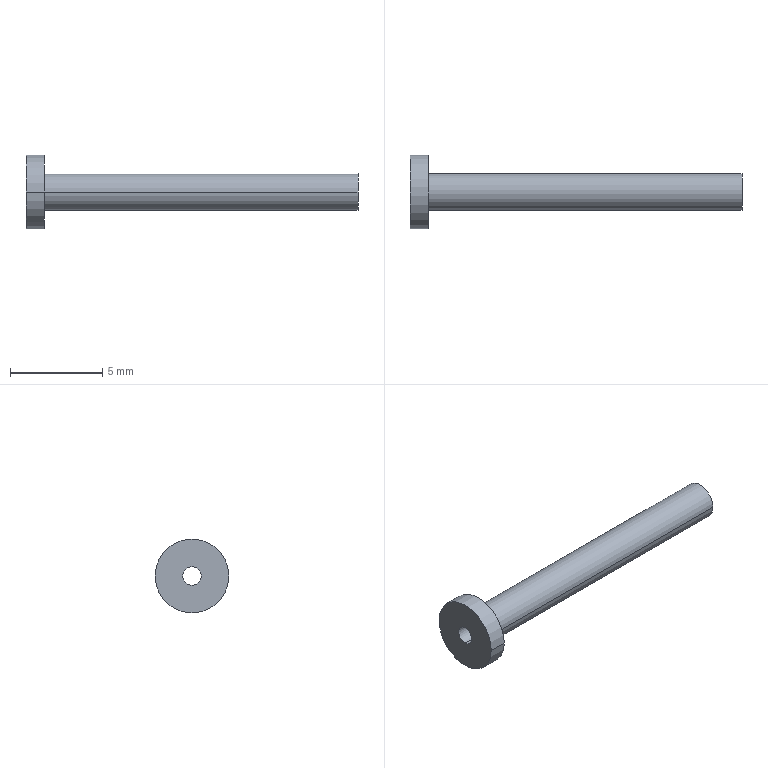Part | STEP file | SKITK4-8 | 1 solid | 9 faces | box 18 x 4 x 4 mm | volume 51.836 mm3 | cylinder 6 | plane 3 | commonest cylinder face diameters 1 x2 2 x2 4 x2
STEP:
#1=CARTESIAN_POINT('',(0.,0.,0.));
#2=DIRECTION('',(0.,0.,1.));
#3=DIRECTION('',(1.,0.,0.));
#4=AXIS2_PLACEMENT_3D('',#1,#2,#3);
#5=CARTESIAN_POINT('',(0.,0.,-0.5));
#6=VERTEX_POINT('',#5);
#7=CARTESIAN_POINT('',(18.,0.,-0.5));
#8=VERTEX_POINT('',#7);
#9=CARTESIAN_POINT('',(0.,0.,-0.5));
#10=DIRECTION('',(1.,0.,0.));
#11=VECTOR('',#10,1.);
#12=LINE('',#9,#11);
#13=CARTESIAN_POINT('',(0.,0.,0.));
#14=DIRECTION('',(1.,0.,0.));
#15=DIRECTION('',(0.,0.,-1.));
#16=AXIS2_PLACEMENT_3D('',#13,#14,#15);
#17=CYLINDRICAL_SURFACE('',#16,0.5);
#18=CARTESIAN_POINT('',(6.283,0.));
#19=DIRECTION('',(0.,1.));
#20=VECTOR('',#19,1.);
#21=LINE('',#18,#20);
#22=(GEOMETRIC_REPRESENTATION_CONTEXT(2)PARAMETRIC_REPRESENTATION_CONTEXT()REPRESENTATION_CONTEXT('',''));
#23=DEFINITIONAL_REPRESENTATION('',(#21),#22);
#24=PCURVE('',#17,#23);
#25=CARTESIAN_POINT('',(0.,0.,0.));
#26=DIRECTION('',(1.,0.,0.));
#27=DIRECTION('',(0.,0.,-1.));
#28=AXIS2_PLACEMENT_3D('',#25,#26,#27);
#29=CYLINDRICAL_SURFACE('',#28,0.5);
#30=CARTESIAN_POINT('',(0.,0.));
#31=DIRECTION('',(0.,1.));
#32=VECTOR('',#31,1.);
#33=LINE('',#30,#32);
#34=(GEOMETRIC_REPRESENTATION_CONTEXT(2)PARAMETRIC_REPRESENTATION_CONTEXT()REPRESENTATION_CONTEXT('',''));
#35=DEFINITIONAL_REPRESENTATION('',(#33),#34);
#36=PCURVE('',#29,#35);
#37=SURFACE_CURVE('',#12,(#24,#36),.PCURVE_S1.);
#38=EDGE_CURVE('',#6,#8,#37,.T.);
#39=ORIENTED_EDGE('',*,*,#38,.T.);
#40=CARTESIAN_POINT('',(18.,0.,0.5));
#41=VERTEX_POINT('',#40);
#42=CARTESIAN_POINT('',(18.,0.,0.));
#43=DIRECTION('',(-1.,0.,0.));
#44=DIRECTION('',(0.,0.,1.));
#45=AXIS2_PLACEMENT_3D('',#42,#43,#44);
#46=CIRCLE('',#45,0.5);
#47=CARTESIAN_POINT('',(9.425,18.));
#48=DIRECTION('',(-1.,0.));
#49=VECTOR('',#48,1.);
#50=LINE('',#47,#49);
#51=(GEOMETRIC_REPRESENTATION_CONTEXT(2)PARAMETRIC_REPRESENTATION_CONTEXT()REPRESENTATION_CONTEXT('',''));
#52=DEFINITIONAL_REPRESENTATION('',(#50),#51);
#53=PCURVE('',#17,#52);
#54=CARTESIAN_POINT('',(18.,0.,0.));
#55=DIRECTION('',(1.,0.,0.));
#56=DIRECTION('',(0.,1.,0.));
#57=AXIS2_PLACEMENT_3D('',#54,#55,#56);
#58=PLANE('',#57);
#59=CARTESIAN_POINT('',(0.,0.5));
#60=CARTESIAN_POINT('',(0.866,0.5));
#61=CARTESIAN_POINT('',(0.433,-0.25));
#62=CARTESIAN_POINT('',(0.,-1.));
#63=CARTESIAN_POINT('',(-0.433,-0.25));
#64=CARTESIAN_POINT('',(-0.866,0.5));
#65=CARTESIAN_POINT('',(0.,0.5));
#66=(BOUNDED_CURVE()B_SPLINE_CURVE(2,(#59,#60,#61,#62,#63,#64,#65),.UNSPECIFIED.,.T.,.F.)B_SPLINE_CURVE_WITH_KNOTS((1,2,2,2,2,1),(-2.094,0.,2.094,4.189,6.283,8.378),.UNSPECIFIED.)CURVE()GEOMETRIC_REPRESENTATION_ITEM()RATIONAL_B_SPLINE_CURVE((1.,0.5,1.,0.5,1.,0.5,1.))REPRESENTATION_ITEM(''));
#67=(GEOMETRIC_REPRESENTATION_CONTEXT(2)PARAMETRIC_REPRESENTATION_CONTEXT()REPRESENTATION_CONTEXT('',''));
#68=DEFINITIONAL_REPRESENTATION('',(#66),#67);
#69=PCURVE('',#58,#68);
#70=SURFACE_CURVE('',#46,(#53,#69),.PCURVE_S1.);
#71=EDGE_CURVE('',#8,#41,#70,.T.);
#72=ORIENTED_EDGE('',*,*,#71,.T.);
#73=CARTESIAN_POINT('',(0.,0.,0.5));
#74=VERTEX_POINT('',#73);
#75=CARTESIAN_POINT('',(0.,0.,0.5));
#76=DIRECTION('',(1.,0.,0.));
#77=VECTOR('',#76,1.);
#78=LINE('',#75,#77);
#79=CARTESIAN_POINT('',(3.142,0.));
#80=DIRECTION('',(0.,1.));
#81=VECTOR('',#80,1.);
#82=LINE('',#79,#81);
#83=(GEOMETRIC_REPRESENTATION_CONTEXT(2)PARAMETRIC_REPRESENTATION_CONTEXT()REPRESENTATION_CONTEXT('',''));
#84=DEFINITIONAL_REPRESENTATION('',(#82),#83);
#85=PCURVE('',#17,#84);
#86=CARTESIAN_POINT('',(3.142,0.));
#87=DIRECTION('',(0.,1.));
#88=VECTOR('',#87,1.);
#89=LINE('',#86,#88);
#90=(GEOMETRIC_REPRESENTATION_CONTEXT(2)PARAMETRIC_REPRESENTATION_CONTEXT()REPRESENTATION_CONTEXT('',''));
#91=DEFINITIONAL_REPRESENTATION('',(#89),#90);
#92=PCURVE('',#29,#91);
#93=SURFACE_CURVE('',#78,(#85,#92),.PCURVE_S1.);
#94=EDGE_CURVE('',#74,#41,#93,.T.);
#95=ORIENTED_EDGE('',*,*,#94,.F.);
#96=CARTESIAN_POINT('',(0.,0.,0.));
#97=DIRECTION('',(1.,0.,0.));
#98=DIRECTION('',(0.,0.,-1.));
#99=AXIS2_PLACEMENT_3D('',#96,#97,#98);
#100=CIRCLE('',#99,0.5);
#101=CARTESIAN_POINT('',(0.,0.));
#102=DIRECTION('',(1.,0.));
#103=VECTOR('',#102,1.);
#104=LINE('',#101,#103);
#105=(GEOMETRIC_REPRESENTATION_CONTEXT(2)PARAMETRIC_REPRESENTATION_CONTEXT()REPRESENTATION_CONTEXT('',''));
#106=DEFINITIONAL_REPRESENTATION('',(#104),#105);
#107=PCURVE('',#17,#106);
#108=CARTESIAN_POINT('',(0.,0.,0.));
#109=DIRECTION('',(-1.,0.,0.));
#110=DIRECTION('',(0.,-1.,0.));
#111=AXIS2_PLACEMENT_3D('',#108,#109,#110);
#112=PLANE('',#111);
#113=CARTESIAN_POINT('',(0.,-0.5));
#114=CARTESIAN_POINT('',(-0.866,-0.5));
#115=CARTESIAN_POINT('',(-0.433,0.25));
#116=CARTESIAN_POINT('',(0.,1.));
#117=CARTESIAN_POINT('',(0.433,0.25));
#118=CARTESIAN_POINT('',(0.866,-0.5));
#119=CARTESIAN_POINT('',(0.,-0.5));
#120=(BOUNDED_CURVE()B_SPLINE_CURVE(2,(#113,#114,#115,#116,#117,#118,#119),.UNSPECIFIED.,.T.,.F.)B_SPLINE_CURVE_WITH_KNOTS((1,2,2,2,2,1),(-2.094,0.,2.094,4.189,6.283,8.378),.UNSPECIFIED.)CURVE()GEOMETRIC_REPRESENTATION_ITEM()RATIONAL_B_SPLINE_CURVE((1.,0.5,1.,0.5,1.,0.5,1.))REPRESENTATION_ITEM(''));
#121=(GEOMETRIC_REPRESENTATION_CONTEXT(2)PARAMETRIC_REPRESENTATION_CONTEXT()REPRESENTATION_CONTEXT('',''));
#122=DEFINITIONAL_REPRESENTATION('',(#120),#121);
#123=PCURVE('',#112,#122);
#124=SURFACE_CURVE('',#100,(#107,#123),.PCURVE_S1.);
#125=EDGE_CURVE('',#74,#6,#124,.T.);
#126=ORIENTED_EDGE('',*,*,#125,.T.);
#127=EDGE_LOOP('',(#39,#72,#95,#126));
#128=FACE_BOUND('',#127,.F.);
#129=ADVANCED_FACE('',(#128),#17,.F.);
#130=CARTESIAN_POINT('',(1.,1.,0.));
#131=VERTEX_POINT('',#130);
#132=CARTESIAN_POINT('',(1.,-1.,0.));
#133=VERTEX_POINT('',#132);
#134=CARTESIAN_POINT('',(1.,0.,0.));
#135=DIRECTION('',(1.,0.,0.));
#136=DIRECTION('',(0.,1.,0.));
#137=AXIS2_PLACEMENT_3D('',#134,#135,#136);
#138=CIRCLE('',#137,1.);
#139=CARTESIAN_POINT('',(1.,0.,0.));
#140=DIRECTION('',(1.,0.,0.));
#141=DIRECTION('',(0.,1.,0.));
#142=AXIS2_PLACEMENT_3D('',#139,#140,#141);
#143=CYLINDRICAL_SURFACE('',#142,1.);
#144=CARTESIAN_POINT('',(0.,0.));
#145=DIRECTION('',(1.,0.));
#146=VECTOR('',#145,1.);
#147=LINE('',#144,#146);
#148=(GEOMETRIC_REPRESENTATION_CONTEXT(2)PARAMETRIC_REPRESENTATION_CONTEXT()REPRESENTATION_CONTEXT('',''));
#149=DEFINITIONAL_REPRESENTATION('',(#147),#148);
#150=PCURVE('',#143,#149);
#151=CARTESIAN_POINT('',(1.,0.,0.));
#152=DIRECTION('',(1.,0.,0.));
#153=DIRECTION('',(0.,1.,0.));
#154=AXIS2_PLACEMENT_3D('',#151,#152,#153);
#155=PLANE('',#154);
#156=CARTESIAN_POINT('',(0.,0.));
#157=DIRECTION('',(1.,0.));
#158=AXIS2_PLACEMENT_2D('',#156,#157);
#159=CIRCLE('',#158,1.);
#160=(GEOMETRIC_REPRESENTATION_CONTEXT(2)PARAMETRIC_REPRESENTATION_CONTEXT()REPRESENTATION_CONTEXT('',''));
#161=DEFINITIONAL_REPRESENTATION('',(#159),#160);
#162=PCURVE('',#155,#161);
#163=SURFACE_CURVE('',#138,(#150,#162),.PCURVE_S1.);
#164=EDGE_CURVE('',#131,#133,#163,.T.);
#165=ORIENTED_EDGE('',*,*,#164,.T.);
#166=CARTESIAN_POINT('',(18.,-1.,0.));
#167=VERTEX_POINT('',#166);
#168=CARTESIAN_POINT('',(1.,-1.,0.));
#169=DIRECTION('',(1.,0.,0.));
#170=VECTOR('',#169,1.);
#171=LINE('',#168,#170);
#172=CARTESIAN_POINT('',(3.142,0.));
#173=DIRECTION('',(0.,1.));
#174=VECTOR('',#173,1.);
#175=LINE('',#172,#174);
#176=(GEOMETRIC_REPRESENTATION_CONTEXT(2)PARAMETRIC_REPRESENTATION_CONTEXT()REPRESENTATION_CONTEXT('',''));
#177=DEFINITIONAL_REPRESENTATION('',(#175),#176);
#178=PCURVE('',#143,#177);
#179=CARTESIAN_POINT('',(1.,0.,0.));
#180=DIRECTION('',(1.,0.,0.));
#181=DIRECTION('',(0.,1.,0.));
#182=AXIS2_PLACEMENT_3D('',#179,#180,#181);
#183=CYLINDRICAL_SURFACE('',#182,1.);
#184=CARTESIAN_POINT('',(3.142,0.));
#185=DIRECTION('',(0.,1.));
#186=VECTOR('',#185,1.);
#187=LINE('',#184,#186);
#188=(GEOMETRIC_REPRESENTATION_CONTEXT(2)PARAMETRIC_REPRESENTATION_CONTEXT()REPRESENTATION_CONTEXT('',''));
#189=DEFINITIONAL_REPRESENTATION('',(#187),#188);
#190=PCURVE('',#183,#189);
#191=SURFACE_CURVE('',#171,(#178,#190),.PCURVE_S1.);
#192=EDGE_CURVE('',#133,#167,#191,.T.);
#193=ORIENTED_EDGE('',*,*,#192,.T.);
#194=CARTESIAN_POINT('',(18.,1.,0.));
#195=VERTEX_POINT('',#194);
#196=CARTESIAN_POINT('',(18.,0.,0.));
#197=DIRECTION('',(-1.,0.,0.));
#198=DIRECTION('',(0.,-1.,0.));
#199=AXIS2_PLACEMENT_3D('',#196,#197,#198);
#200=CIRCLE('',#199,1.);
#201=CARTESIAN_POINT('',(3.142,17.));
#202=DIRECTION('',(-1.,0.));
#203=VECTOR('',#202,1.);
#204=LINE('',#201,#203);
#205=(GEOMETRIC_REPRESENTATION_CONTEXT(2)PARAMETRIC_REPRESENTATION_CONTEXT()REPRESENTATION_CONTEXT('',''));
#206=DEFINITIONAL_REPRESENTATION('',(#204),#205);
#207=PCURVE('',#143,#206);
#208=CARTESIAN_POINT('',(-1.,0.));
#209=CARTESIAN_POINT('',(-1.,1.732));
#210=CARTESIAN_POINT('',(0.5,0.866));
#211=CARTESIAN_POINT('',(2.,0.));
#212=CARTESIAN_POINT('',(0.5,-0.866));
#213=CARTESIAN_POINT('',(-1.,-1.732));
#214=CARTESIAN_POINT('',(-1.,0.));
#215=(BOUNDED_CURVE()B_SPLINE_CURVE(2,(#208,#209,#210,#211,#212,#213,#214),.UNSPECIFIED.,.T.,.F.)B_SPLINE_CURVE_WITH_KNOTS((1,2,2,2,2,1),(-2.094,0.,2.094,4.189,6.283,8.378),.UNSPECIFIED.)CURVE()GEOMETRIC_REPRESENTATION_ITEM()RATIONAL_B_SPLINE_CURVE((1.,0.5,1.,0.5,1.,0.5,1.))REPRESENTATION_ITEM(''));
#216=(GEOMETRIC_REPRESENTATION_CONTEXT(2)PARAMETRIC_REPRESENTATION_CONTEXT()REPRESENTATION_CONTEXT('',''));
#217=DEFINITIONAL_REPRESENTATION('',(#215),#216);
#218=PCURVE('',#58,#217);
#219=SURFACE_CURVE('',#200,(#207,#218),.PCURVE_S1.);
#220=EDGE_CURVE('',#167,#195,#219,.T.);
#221=ORIENTED_EDGE('',*,*,#220,.T.);
#222=CARTESIAN_POINT('',(1.,1.,0.));
#223=DIRECTION('',(1.,0.,0.));
#224=VECTOR('',#223,1.);
#225=LINE('',#222,#224);
#226=CARTESIAN_POINT('',(0.,0.));
#227=DIRECTION('',(0.,1.));
#228=VECTOR('',#227,1.);
#229=LINE('',#226,#228);
#230=(GEOMETRIC_REPRESENTATION_CONTEXT(2)PARAMETRIC_REPRESENTATION_CONTEXT()REPRESENTATION_CONTEXT('',''));
#231=DEFINITIONAL_REPRESENTATION('',(#229),#230);
#232=PCURVE('',#143,#231);
#233=CARTESIAN_POINT('',(6.283,0.));
#234=DIRECTION('',(0.,1.));
#235=VECTOR('',#234,1.);
#236=LINE('',#233,#235);
#237=(GEOMETRIC_REPRESENTATION_CONTEXT(2)PARAMETRIC_REPRESENTATION_CONTEXT()REPRESENTATION_CONTEXT('',''));
#238=DEFINITIONAL_REPRESENTATION('',(#236),#237);
#239=PCURVE('',#183,#238);
#240=SURFACE_CURVE('',#225,(#232,#239),.PCURVE_S1.);
#241=EDGE_CURVE('',#131,#195,#240,.T.);
#242=ORIENTED_EDGE('',*,*,#241,.F.);
#243=EDGE_LOOP('',(#165,#193,#221,#242));
#244=FACE_BOUND('',#243,.T.);
#245=ADVANCED_FACE('',(#244),#143,.T.);
#246=CARTESIAN_POINT('',(0.,2.,0.));
#247=VERTEX_POINT('',#246);
#248=CARTESIAN_POINT('',(0.,-2.,0.));
#249=VERTEX_POINT('',#248);
#250=CARTESIAN_POINT('',(0.,0.,0.));
#251=DIRECTION('',(1.,0.,0.));
#252=DIRECTION('',(0.,1.,0.));
#253=AXIS2_PLACEMENT_3D('',#250,#251,#252);
#254=CIRCLE('',#253,2.);
#255=CARTESIAN_POINT('',(0.,0.,0.));
#256=DIRECTION('',(1.,0.,0.));
#257=DIRECTION('',(0.,1.,0.));
#258=AXIS2_PLACEMENT_3D('',#255,#256,#257);
#259=CYLINDRICAL_SURFACE('',#258,2.);
#260=CARTESIAN_POINT('',(0.,0.));
#261=DIRECTION('',(1.,0.));
#262=VECTOR('',#261,1.);
#263=LINE('',#260,#262);
#264=(GEOMETRIC_REPRESENTATION_CONTEXT(2)PARAMETRIC_REPRESENTATION_CONTEXT()REPRESENTATION_CONTEXT('',''));
#265=DEFINITIONAL_REPRESENTATION('',(#263),#264);
#266=PCURVE('',#259,#265);
#267=CARTESIAN_POINT('',(-2.,0.));
#268=CARTESIAN_POINT('',(-2.,3.464));
#269=CARTESIAN_POINT('',(1.,1.732));
#270=CARTESIAN_POINT('',(4.,0.));
#271=CARTESIAN_POINT('',(1.,-1.732));
#272=CARTESIAN_POINT('',(-2.,-3.464));
#273=CARTESIAN_POINT('',(-2.,0.));
#274=(BOUNDED_CURVE()B_SPLINE_CURVE(2,(#267,#268,#269,#270,#271,#272,#273),.UNSPECIFIED.,.T.,.F.)B_SPLINE_CURVE_WITH_KNOTS((1,2,2,2,2,1),(-2.094,0.,2.094,4.189,6.283,8.378),.UNSPECIFIED.)CURVE()GEOMETRIC_REPRESENTATION_ITEM()RATIONAL_B_SPLINE_CURVE((1.,0.5,1.,0.5,1.,0.5,1.))REPRESENTATION_ITEM(''));
#275=(GEOMETRIC_REPRESENTATION_CONTEXT(2)PARAMETRIC_REPRESENTATION_CONTEXT()REPRESENTATION_CONTEXT('',''));
#276=DEFINITIONAL_REPRESENTATION('',(#274),#275);
#277=PCURVE('',#112,#276);
#278=SURFACE_CURVE('',#254,(#266,#277),.PCURVE_S1.);
#279=EDGE_CURVE('',#247,#249,#278,.T.);
#280=ORIENTED_EDGE('',*,*,#279,.T.);
#281=CARTESIAN_POINT('',(1.,-2.,0.));
#282=VERTEX_POINT('',#281);
#283=CARTESIAN_POINT('',(0.,-2.,0.));
#284=DIRECTION('',(1.,0.,0.));
#285=VECTOR('',#284,1.);
#286=LINE('',#283,#285);
#287=CARTESIAN_POINT('',(3.142,0.));
#288=DIRECTION('',(0.,1.));
#289=VECTOR('',#288,1.);
#290=LINE('',#287,#289);
#291=(GEOMETRIC_REPRESENTATION_CONTEXT(2)PARAMETRIC_REPRESENTATION_CONTEXT()REPRESENTATION_CONTEXT('',''));
#292=DEFINITIONAL_REPRESENTATION('',(#290),#291);
#293=PCURVE('',#259,#292);
#294=CARTESIAN_POINT('',(0.,0.,0.));
#295=DIRECTION('',(1.,0.,0.));
#296=DIRECTION('',(0.,1.,0.));
#297=AXIS2_PLACEMENT_3D('',#294,#295,#296);
#298=CYLINDRICAL_SURFACE('',#297,2.);
#299=CARTESIAN_POINT('',(3.142,0.));
#300=DIRECTION('',(0.,1.));
#301=VECTOR('',#300,1.);
#302=LINE('',#299,#301);
#303=(GEOMETRIC_REPRESENTATION_CONTEXT(2)PARAMETRIC_REPRESENTATION_CONTEXT()REPRESENTATION_CONTEXT('',''));
#304=DEFINITIONAL_REPRESENTATION('',(#302),#303);
#305=PCURVE('',#298,#304);
#306=SURFACE_CURVE('',#286,(#293,#305),.PCURVE_S1.);
#307=EDGE_CURVE('',#249,#282,#306,.T.);
#308=ORIENTED_EDGE('',*,*,#307,.T.);
#309=CARTESIAN_POINT('',(1.,2.,0.));
#310=VERTEX_POINT('',#309);
#311=CARTESIAN_POINT('',(1.,0.,0.));
#312=DIRECTION('',(-1.,0.,0.));
#313=DIRECTION('',(0.,-1.,0.));
#314=AXIS2_PLACEMENT_3D('',#311,#312,#313);
#315=CIRCLE('',#314,2.);
#316=CARTESIAN_POINT('',(3.142,1.));
#317=DIRECTION('',(-1.,0.));
#318=VECTOR('',#317,1.);
#319=LINE('',#316,#318);
#320=(GEOMETRIC_REPRESENTATION_CONTEXT(2)PARAMETRIC_REPRESENTATION_CONTEXT()REPRESENTATION_CONTEXT('',''));
#321=DEFINITIONAL_REPRESENTATION('',(#319),#320);
#322=PCURVE('',#259,#321);
#323=CARTESIAN_POINT('',(-2.,0.));
#324=CARTESIAN_POINT('',(-2.,3.464));
#325=CARTESIAN_POINT('',(1.,1.732));
#326=CARTESIAN_POINT('',(4.,0.));
#327=CARTESIAN_POINT('',(1.,-1.732));
#328=CARTESIAN_POINT('',(-2.,-3.464));
#329=CARTESIAN_POINT('',(-2.,0.));
#330=(BOUNDED_CURVE()B_SPLINE_CURVE(2,(#323,#324,#325,#326,#327,#328,#329),.UNSPECIFIED.,.T.,.F.)B_SPLINE_CURVE_WITH_KNOTS((1,2,2,2,2,1),(-2.094,0.,2.094,4.189,6.283,8.378),.UNSPECIFIED.)CURVE()GEOMETRIC_REPRESENTATION_ITEM()RATIONAL_B_SPLINE_CURVE((1.,0.5,1.,0.5,1.,0.5,1.))REPRESENTATION_ITEM(''));
#331=(GEOMETRIC_REPRESENTATION_CONTEXT(2)PARAMETRIC_REPRESENTATION_CONTEXT()REPRESENTATION_CONTEXT('',''));
#332=DEFINITIONAL_REPRESENTATION('',(#330),#331);
#333=PCURVE('',#155,#332);
#334=SURFACE_CURVE('',#315,(#322,#333),.PCURVE_S1.);
#335=EDGE_CURVE('',#282,#310,#334,.T.);
#336=ORIENTED_EDGE('',*,*,#335,.T.);
#337=CARTESIAN_POINT('',(0.,2.,0.));
#338=DIRECTION('',(1.,0.,0.));
#339=VECTOR('',#338,1.);
#340=LINE('',#337,#339);
#341=CARTESIAN_POINT('',(0.,0.));
#342=DIRECTION('',(0.,1.));
#343=VECTOR('',#342,1.);
#344=LINE('',#341,#343);
#345=(GEOMETRIC_REPRESENTATION_CONTEXT(2)PARAMETRIC_REPRESENTATION_CONTEXT()REPRESENTATION_CONTEXT('',''));
#346=DEFINITIONAL_REPRESENTATION('',(#344),#345);
#347=PCURVE('',#259,#346);
#348=CARTESIAN_POINT('',(6.283,0.));
#349=DIRECTION('',(0.,1.));
#350=VECTOR('',#349,1.);
#351=LINE('',#348,#350);
#352=(GEOMETRIC_REPRESENTATION_CONTEXT(2)PARAMETRIC_REPRESENTATION_CONTEXT()REPRESENTATION_CONTEXT('',''));
#353=DEFINITIONAL_REPRESENTATION('',(#351),#352);
#354=PCURVE('',#298,#353);
#355=SURFACE_CURVE('',#340,(#347,#354),.PCURVE_S1.);
#356=EDGE_CURVE('',#247,#310,#355,.T.);
#357=ORIENTED_EDGE('',*,*,#356,.F.);
#358=EDGE_LOOP('',(#280,#308,#336,#357));
#359=FACE_BOUND('',#358,.T.);
#360=ADVANCED_FACE('',(#359),#259,.T.);
#361=ORIENTED_EDGE('',*,*,#164,.F.);
#362=CARTESIAN_POINT('',(1.,0.,0.));
#363=DIRECTION('',(1.,0.,0.));
#364=DIRECTION('',(0.,1.,0.));
#365=AXIS2_PLACEMENT_3D('',#362,#363,#364);
#366=CIRCLE('',#365,1.);
#367=CARTESIAN_POINT('',(0.,0.));
#368=DIRECTION('',(1.,0.));
#369=AXIS2_PLACEMENT_2D('',#367,#368);
#370=CIRCLE('',#369,1.);
#371=(GEOMETRIC_REPRESENTATION_CONTEXT(2)PARAMETRIC_REPRESENTATION_CONTEXT()REPRESENTATION_CONTEXT('',''));
#372=DEFINITIONAL_REPRESENTATION('',(#370),#371);
#373=PCURVE('',#155,#372);
#374=CARTESIAN_POINT('',(0.,0.));
#375=DIRECTION('',(1.,0.));
#376=VECTOR('',#375,1.);
#377=LINE('',#374,#376);
#378=(GEOMETRIC_REPRESENTATION_CONTEXT(2)PARAMETRIC_REPRESENTATION_CONTEXT()REPRESENTATION_CONTEXT('',''));
#379=DEFINITIONAL_REPRESENTATION('',(#377),#378);
#380=PCURVE('',#183,#379);
#381=SURFACE_CURVE('',#366,(#373,#380),.PCURVE_S1.);
#382=EDGE_CURVE('',#133,#131,#381,.T.);
#383=ORIENTED_EDGE('',*,*,#382,.F.);
#384=EDGE_LOOP('',(#361,#383));
#385=FACE_BOUND('',#384,.T.);
#386=CARTESIAN_POINT('',(1.,0.,0.));
#387=DIRECTION('',(-1.,0.,0.));
#388=DIRECTION('',(0.,-1.,0.));
#389=AXIS2_PLACEMENT_3D('',#386,#387,#388);
#390=CIRCLE('',#389,2.);
#391=CARTESIAN_POINT('',(-2.,0.));
#392=CARTESIAN_POINT('',(-2.,3.464));
#393=CARTESIAN_POINT('',(1.,1.732));
#394=CARTESIAN_POINT('',(4.,0.));
#395=CARTESIAN_POINT('',(1.,-1.732));
#396=CARTESIAN_POINT('',(-2.,-3.464));
#397=CARTESIAN_POINT('',(-2.,0.));
#398=(BOUNDED_CURVE()B_SPLINE_CURVE(2,(#391,#392,#393,#394,#395,#396,#397),.UNSPECIFIED.,.T.,.F.)B_SPLINE_CURVE_WITH_KNOTS((1,2,2,2,2,1),(-2.094,0.,2.094,4.189,6.283,8.378),.UNSPECIFIED.)CURVE()GEOMETRIC_REPRESENTATION_ITEM()RATIONAL_B_SPLINE_CURVE((1.,0.5,1.,0.5,1.,0.5,1.))REPRESENTATION_ITEM(''));
#399=(GEOMETRIC_REPRESENTATION_CONTEXT(2)PARAMETRIC_REPRESENTATION_CONTEXT()REPRESENTATION_CONTEXT('',''));
#400=DEFINITIONAL_REPRESENTATION('',(#398),#399);
#401=PCURVE('',#155,#400);
#402=CARTESIAN_POINT('',(9.425,1.));
#403=DIRECTION('',(-1.,0.));
#404=VECTOR('',#403,1.);
#405=LINE('',#402,#404);
#406=(GEOMETRIC_REPRESENTATION_CONTEXT(2)PARAMETRIC_REPRESENTATION_CONTEXT()REPRESENTATION_CONTEXT('',''));
#407=DEFINITIONAL_REPRESENTATION('',(#405),#406);
#408=PCURVE('',#298,#407);
#409=SURFACE_CURVE('',#390,(#401,#408),.PCURVE_S1.);
#410=EDGE_CURVE('',#310,#282,#409,.T.);
#411=ORIENTED_EDGE('',*,*,#410,.F.);
#412=ORIENTED_EDGE('',*,*,#335,.F.);
#413=EDGE_LOOP('',(#411,#412));
#414=FACE_BOUND('',#413,.T.);
#415=ADVANCED_FACE('',(#385,#414),#155,.T.);
#416=CARTESIAN_POINT('',(0.,0.,0.));
#417=DIRECTION('',(1.,0.,0.));
#418=DIRECTION('',(0.,0.,-1.));
#419=AXIS2_PLACEMENT_3D('',#416,#417,#418);
#420=CIRCLE('',#419,0.5);
#421=CARTESIAN_POINT('',(0.,-0.5));
#422=CARTESIAN_POINT('',(-0.866,-0.5));
#423=CARTESIAN_POINT('',(-0.433,0.25));
#424=CARTESIAN_POINT('',(0.,1.));
#425=CARTESIAN_POINT('',(0.433,0.25));
#426=CARTESIAN_POINT('',(0.866,-0.5));
#427=CARTESIAN_POINT('',(0.,-0.5));
#428=(BOUNDED_CURVE()B_SPLINE_CURVE(2,(#421,#422,#423,#424,#425,#426,#427),.UNSPECIFIED.,.T.,.F.)B_SPLINE_CURVE_WITH_KNOTS((1,2,2,2,2,1),(-2.094,0.,2.094,4.189,6.283,8.378),.UNSPECIFIED.)CURVE()GEOMETRIC_REPRESENTATION_ITEM()RATIONAL_B_SPLINE_CURVE((1.,0.5,1.,0.5,1.,0.5,1.))REPRESENTATION_ITEM(''));
#429=(GEOMETRIC_REPRESENTATION_CONTEXT(2)PARAMETRIC_REPRESENTATION_CONTEXT()REPRESENTATION_CONTEXT('',''));
#430=DEFINITIONAL_REPRESENTATION('',(#428),#429);
#431=PCURVE('',#112,#430);
#432=CARTESIAN_POINT('',(0.,0.));
#433=DIRECTION('',(1.,0.));
#434=VECTOR('',#433,1.);
#435=LINE('',#432,#434);
#436=(GEOMETRIC_REPRESENTATION_CONTEXT(2)PARAMETRIC_REPRESENTATION_CONTEXT()REPRESENTATION_CONTEXT('',''));
#437=DEFINITIONAL_REPRESENTATION('',(#435),#436);
#438=PCURVE('',#29,#437);
#439=SURFACE_CURVE('',#420,(#431,#438),.PCURVE_S1.);
#440=EDGE_CURVE('',#6,#74,#439,.T.);
#441=ORIENTED_EDGE('',*,*,#440,.T.);
#442=ORIENTED_EDGE('',*,*,#125,.T.);
#443=EDGE_LOOP('',(#441,#442));
#444=FACE_BOUND('',#443,.T.);
#445=ORIENTED_EDGE('',*,*,#279,.F.);
#446=CARTESIAN_POINT('',(0.,0.,0.));
#447=DIRECTION('',(1.,0.,0.));
#448=DIRECTION('',(0.,1.,0.));
#449=AXIS2_PLACEMENT_3D('',#446,#447,#448);
#450=CIRCLE('',#449,2.);
#451=CARTESIAN_POINT('',(-2.,0.));
#452=CARTESIAN_POINT('',(-2.,3.464));
#453=CARTESIAN_POINT('',(1.,1.732));
#454=CARTESIAN_POINT('',(4.,0.));
#455=CARTESIAN_POINT('',(1.,-1.732));
#456=CARTESIAN_POINT('',(-2.,-3.464));
#457=CARTESIAN_POINT('',(-2.,0.));
#458=(BOUNDED_CURVE()B_SPLINE_CURVE(2,(#451,#452,#453,#454,#455,#456,#457),.UNSPECIFIED.,.T.,.F.)B_SPLINE_CURVE_WITH_KNOTS((1,2,2,2,2,1),(-2.094,0.,2.094,4.189,6.283,8.378),.UNSPECIFIED.)CURVE()GEOMETRIC_REPRESENTATION_ITEM()RATIONAL_B_SPLINE_CURVE((1.,0.5,1.,0.5,1.,0.5,1.))REPRESENTATION_ITEM(''));
#459=(GEOMETRIC_REPRESENTATION_CONTEXT(2)PARAMETRIC_REPRESENTATION_CONTEXT()REPRESENTATION_CONTEXT('',''));
#460=DEFINITIONAL_REPRESENTATION('',(#458),#459);
#461=PCURVE('',#112,#460);
#462=CARTESIAN_POINT('',(0.,0.));
#463=DIRECTION('',(1.,0.));
#464=VECTOR('',#463,1.);
#465=LINE('',#462,#464);
#466=(GEOMETRIC_REPRESENTATION_CONTEXT(2)PARAMETRIC_REPRESENTATION_CONTEXT()REPRESENTATION_CONTEXT('',''));
#467=DEFINITIONAL_REPRESENTATION('',(#465),#466);
#468=PCURVE('',#298,#467);
#469=SURFACE_CURVE('',#450,(#461,#468),.PCURVE_S1.);
#470=EDGE_CURVE('',#249,#247,#469,.T.);
#471=ORIENTED_EDGE('',*,*,#470,.F.);
#472=EDGE_LOOP('',(#445,#471));
#473=FACE_BOUND('',#472,.T.);
#474=ADVANCED_FACE('',(#444,#473),#112,.T.);
#475=ORIENTED_EDGE('',*,*,#307,.F.);
#476=ORIENTED_EDGE('',*,*,#470,.T.);
#477=ORIENTED_EDGE('',*,*,#356,.T.);
#478=ORIENTED_EDGE('',*,*,#410,.T.);
#479=EDGE_LOOP('',(#475,#476,#477,#478));
#480=FACE_BOUND('',#479,.T.);
#481=ADVANCED_FACE('',(#480),#298,.T.);
#482=ORIENTED_EDGE('',*,*,#71,.T.);
#483=CARTESIAN_POINT('',(18.,0.,0.));
#484=DIRECTION('',(-1.,0.,0.));
#485=DIRECTION('',(0.,0.,1.));
#486=AXIS2_PLACEMENT_3D('',#483,#484,#485);
#487=CIRCLE('',#486,0.5);
#488=CARTESIAN_POINT('',(0.,0.5));
#489=CARTESIAN_POINT('',(0.866,0.5));
#490=CARTESIAN_POINT('',(0.433,-0.25));
#491=CARTESIAN_POINT('',(0.,-1.));
#492=CARTESIAN_POINT('',(-0.433,-0.25));
#493=CARTESIAN_POINT('',(-0.866,0.5));
#494=CARTESIAN_POINT('',(0.,0.5));
#495=(BOUNDED_CURVE()B_SPLINE_CURVE(2,(#488,#489,#490,#491,#492,#493,#494),.UNSPECIFIED.,.T.,.F.)B_SPLINE_CURVE_WITH_KNOTS((1,2,2,2,2,1),(-2.094,0.,2.094,4.189,6.283,8.378),.UNSPECIFIED.)CURVE()GEOMETRIC_REPRESENTATION_ITEM()RATIONAL_B_SPLINE_CURVE((1.,0.5,1.,0.5,1.,0.5,1.))REPRESENTATION_ITEM(''));
#496=(GEOMETRIC_REPRESENTATION_CONTEXT(2)PARAMETRIC_REPRESENTATION_CONTEXT()REPRESENTATION_CONTEXT('',''));
#497=DEFINITIONAL_REPRESENTATION('',(#495),#496);
#498=PCURVE('',#58,#497);
#499=CARTESIAN_POINT('',(3.142,18.));
#500=DIRECTION('',(-1.,0.));
#501=VECTOR('',#500,1.);
#502=LINE('',#499,#501);
#503=(GEOMETRIC_REPRESENTATION_CONTEXT(2)PARAMETRIC_REPRESENTATION_CONTEXT()REPRESENTATION_CONTEXT('',''));
#504=DEFINITIONAL_REPRESENTATION('',(#502),#503);
#505=PCURVE('',#29,#504);
#506=SURFACE_CURVE('',#487,(#498,#505),.PCURVE_S1.);
#507=EDGE_CURVE('',#41,#8,#506,.T.);
#508=ORIENTED_EDGE('',*,*,#507,.T.);
#509=EDGE_LOOP('',(#482,#508));
#510=FACE_BOUND('',#509,.T.);
#511=CARTESIAN_POINT('',(18.,0.,0.));
#512=DIRECTION('',(-1.,0.,0.));
#513=DIRECTION('',(0.,-1.,0.));
#514=AXIS2_PLACEMENT_3D('',#511,#512,#513);
#515=CIRCLE('',#514,1.);
#516=CARTESIAN_POINT('',(-1.,0.));
#517=CARTESIAN_POINT('',(-1.,1.732));
#518=CARTESIAN_POINT('',(0.5,0.866));
#519=CARTESIAN_POINT('',(2.,0.));
#520=CARTESIAN_POINT('',(0.5,-0.866));
#521=CARTESIAN_POINT('',(-1.,-1.732));
#522=CARTESIAN_POINT('',(-1.,0.));
#523=(BOUNDED_CURVE()B_SPLINE_CURVE(2,(#516,#517,#518,#519,#520,#521,#522),.UNSPECIFIED.,.T.,.F.)B_SPLINE_CURVE_WITH_KNOTS((1,2,2,2,2,1),(-2.094,0.,2.094,4.189,6.283,8.378),.UNSPECIFIED.)CURVE()GEOMETRIC_REPRESENTATION_ITEM()RATIONAL_B_SPLINE_CURVE((1.,0.5,1.,0.5,1.,0.5,1.))REPRESENTATION_ITEM(''));
#524=(GEOMETRIC_REPRESENTATION_CONTEXT(2)PARAMETRIC_REPRESENTATION_CONTEXT()REPRESENTATION_CONTEXT('',''));
#525=DEFINITIONAL_REPRESENTATION('',(#523),#524);
#526=PCURVE('',#58,#525);
#527=CARTESIAN_POINT('',(9.425,17.));
#528=DIRECTION('',(-1.,0.));
#529=VECTOR('',#528,1.);
#530=LINE('',#527,#529);
#531=(GEOMETRIC_REPRESENTATION_CONTEXT(2)PARAMETRIC_REPRESENTATION_CONTEXT()REPRESENTATION_CONTEXT('',''));
#532=DEFINITIONAL_REPRESENTATION('',(#530),#531);
#533=PCURVE('',#183,#532);
#534=SURFACE_CURVE('',#515,(#526,#533),.PCURVE_S1.);
#535=EDGE_CURVE('',#195,#167,#534,.T.);
#536=ORIENTED_EDGE('',*,*,#535,.F.);
#537=ORIENTED_EDGE('',*,*,#220,.F.);
#538=EDGE_LOOP('',(#536,#537));
#539=FACE_BOUND('',#538,.T.);
#540=ADVANCED_FACE('',(#510,#539),#58,.T.);
#541=ORIENTED_EDGE('',*,*,#192,.F.);
#542=ORIENTED_EDGE('',*,*,#382,.T.);
#543=ORIENTED_EDGE('',*,*,#241,.T.);
#544=ORIENTED_EDGE('',*,*,#535,.T.);
#545=EDGE_LOOP('',(#541,#542,#543,#544));
#546=FACE_BOUND('',#545,.T.);
#547=ADVANCED_FACE('',(#546),#183,.T.);
#548=ORIENTED_EDGE('',*,*,#507,.T.);
#549=ORIENTED_EDGE('',*,*,#38,.F.);
#550=ORIENTED_EDGE('',*,*,#440,.T.);
#551=ORIENTED_EDGE('',*,*,#94,.T.);
#552=EDGE_LOOP('',(#548,#549,#550,#551));
#553=FACE_BOUND('',#552,.F.);
#554=ADVANCED_FACE('',(#553),#29,.F.);
#555=CLOSED_SHELL('',(#129,#245,#360,#415,#474,#481,#540,#547,#554));
#556=MANIFOLD_SOLID_BREP('',#555);
#557=(LENGTH_UNIT()NAMED_UNIT(*)SI_UNIT(.MILLI.,.METRE.));
#558=UNCERTAINTY_MEASURE_WITH_UNIT(LENGTH_MEASURE(0.0000001),#557,'','');
#559=(NAMED_UNIT(*)PLANE_ANGLE_UNIT()SI_UNIT($,.RADIAN.));
#560=(NAMED_UNIT(*)SI_UNIT($,.STERADIAN.)SOLID_ANGLE_UNIT());
#561=(GEOMETRIC_REPRESENTATION_CONTEXT(3)GLOBAL_UNCERTAINTY_ASSIGNED_CONTEXT((#558))GLOBAL_UNIT_ASSIGNED_CONTEXT((#557,#559,#560))REPRESENTATION_CONTEXT('',''));
#562=ADVANCED_BREP_SHAPE_REPRESENTATION('',(#4,#556),#561);